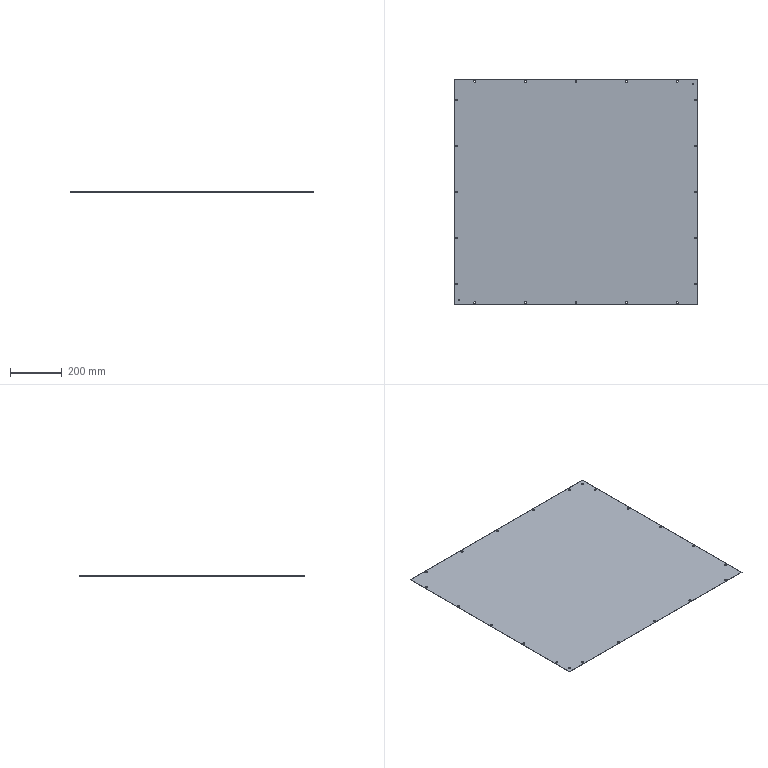Part | 1 solid | 100 faces | box 940 x 870 x 1 mm | volume 816571 mm3 | cylinder 54 | plane 46 | commonest cylinder face diameters 7 x50 5 x4